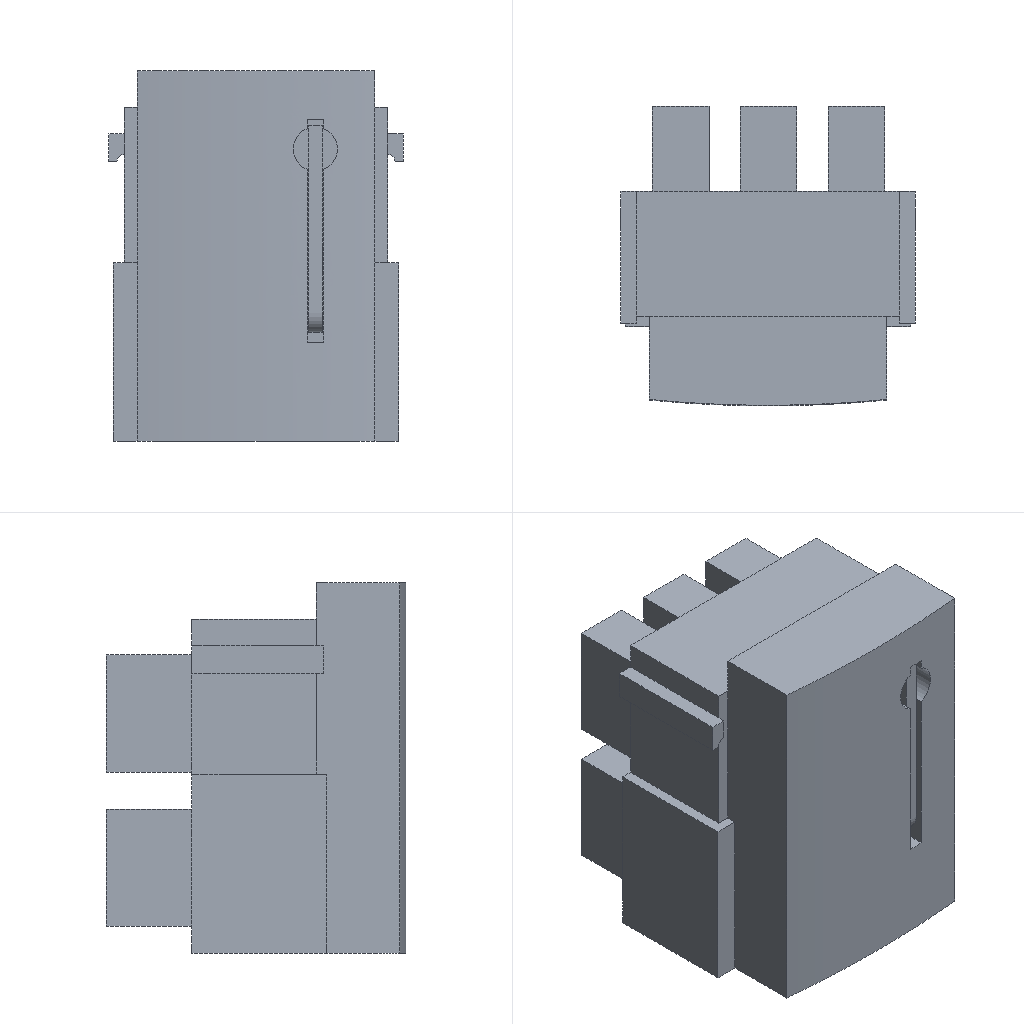Simulation study | abaqus
Set-up summary:
category,name,step,type,value,unit,region
solver,abaqus,,Abaqus/CAE 2024
units,mm-N-s-tonne (MPa),,inferred,E=200000 density=7.8e-09
analysis,Step-1,,dynamic implicit,time_period=0.02
analysis,Step-2,,dynamic implicit,time_period=0.02
mesh,nodes,,,214940
mesh,elements,,,173322
element_type,C3D8R,,,173322
material,Q235,,E,200000
material,Q235,,nu,0.3
material,Q235,,density,7.8e-09
material,Q235,,behaviors,damping
section,Q235,,solid section,,,_PickedSet41
bc,BC-1,initial,encastre,[dofs=ENCASTRE],,_PickedSet4
bc,BC-2,Step-1,acceleration,"-1 [dofs=rx,ry,rz,x,y,z n=6]",,_PickedSet14
bc,BC-1,Step-2,encastre,[dofs=ENCASTRE],,_PickedSet4
Abaqus input file, long lists of numbers shortened:
*Heading
** Job name: deck Model name: 0428-Copy
** Generated by: Abaqus/CAE 2024
*Preprint, echo=NO, model=NO, history=NO, contact=NO
**
** PARTS
**
*Part, name=duanluqi
*Node
      1,   188.98,           0.,   78.818
      2,   188.98,         16.5,   78.818
** (214938 more lines like these left out)
*Element, type=C3D8R
   1,    564,  12340,  99771,  10843,      1,    360,  10483,    396
   2,  12340,  12341,  99772,  99771,    360,    361,  10484,  10483
** (173320 more lines like these left out)
*Nset, nset=_PickedSet41, internal, generate
      1,  214940,       1
*Elset, elset=_PickedSet41, internal, generate
      1,  173322,       1
** Section: Section-1
*Solid Section, elset=_PickedSet41, material=Q235
,
*End Part
**
**
** ASSEMBLY
**
*Assembly, name=Assembly
**
*Instance, name=duanluqi-1, part=duanluqi
*End Instance
**
*Nset, nset=_PickedSet4, internal, instance=duanluqi-1
    10,    11,    12,    13,    19,    22,    47,    48,   109,   110,   113,   115,   116,   117,   441,   442
   443,   444,   445,   446,   447,   448,   449,   450,   451,   452,   453,   454,   455,   456,   457,   458
** (262 more lines like these left out)
*Elset, elset=_PickedSet4, internal, instance=duanluqi-1
  5601,  5602,  5603,  5604,  5605,  5606,  5607,  5608,  5609,  5610,  5611,  5612,  5613,  5614,  5615,  5616
  5617,  5618,  5619,  5620,  5621,  5622,  5623,  5624,  5625,  5626,  5627,  5628,  5629,  5630,  5631,  5632
** (253 more lines like these left out)
*Nset, nset=_PickedSet14, internal, instance=duanluqi-1
    26,    27,    40,    41,    43,   319,   320,  1240,  1241,  1242,  1243,  1244,  1245,  1246,  1247,  1248
  1249,  1250,  1251,  1252,  1253,  1254,  1255,  1256,  1257,  1258,  1259,  1260,  1261,  1262,  1263,  1264
** (55 more lines like these left out)
*Elset, elset=_PickedSet14, internal, instance=duanluqi-1
  29009,  29010,  29011,  29012,  29013,  29014,  29015,  29016,  29017,  29018,  29019,  29020,  29021,  29022,  29023,  29024
  29025,  29026,  29027,  29028,  29029,  29030,  29031,  29032,  29033,  29034,  29035,  29036,  29037,  29038,  29039,  29040
** (50 more lines like these left out)
*Elset, elset=__PickedSurf12_S4, internal, instance=duanluqi-1
   5922,   6020,   6118,   6216,   6314,   6412,   6510,   6608,   6706,   6804,   6902,   7000,   7098,   7196,   7294,   7392
   7490,   7588,   7686,   7784,   7882,   7980,   8078,   8176,   8274,   8372,   8470,   8568,   8666,   8764,   8862,   8960
** (26 more lines like these left out)
*Elset, elset=__PickedSurf12_S2, internal, instance=duanluqi-1
 127371, 127372, 127373, 127374, 127375, 127376, 127377, 127378, 127379, 127380, 127381, 127382, 127383, 127384, 127385, 127386
 127387, 127388, 127389, 127390, 127391, 127392, 127393, 127394, 127395, 127396, 127397, 127398, 127399, 127400, 127401, 127402
** (54 more lines like these left out)
*Elset, elset=__PickedSurf12_S5, internal, instance=duanluqi-1
 29009, 29010, 29011, 29012, 29013, 29014, 29015, 29016, 29017, 29018, 29019, 29020, 29021, 29022, 29023, 29024
 29025, 29026, 29027, 29028, 29029, 29030, 29031, 29032, 29033, 29034, 29035, 29036, 29037, 29038, 29039, 29040
** (10 more lines like these left out)
*Surface, type=ELEMENT, name=_PickedSurf12, internal
__PickedSurf12_S4, S4
__PickedSurf12_S2, S2
__PickedSurf12_S5, S5
*End Assembly
*Amplitude, name=Amp-1
             0.,              0.,          0.0057,              0.,           0.019,         392000.,          0.0191,              0.
           0.02,              0.
**
** MATERIALS
**
*Material, name=Q235
*Damping, alpha=0.3132, beta=7.94e-06
*Density
 7.8e-09,
*Elastic
200000., 0.3
**
** INTERACTION PROPERTIES
**
*Surface Interaction, name=IntProp-1
1.,
*Friction, slip tolerance=0.005
 0.1,
*Surface Behavior, pressure-overclosure=HARD
**
** BOUNDARY CONDITIONS
**
** Name: BC-1 Type: Symmetry/Antisymmetry/Encastre
*Boundary
_PickedSet4, ENCASTRE
** ----------------------------------------------------------------
**
** STEP: Step-1
**
*Step, name=Step-1, nlgeom=NO, inc=1000
*Dynamic
0.002,0.02,2e-07
**
** BOUNDARY CONDITIONS
**
** Name: BC-2 Type: Acceleration/Angular acceleration
*Boundary, amplitude=Amp-1, type=ACCELERATION
_PickedSet14, 1, 1
_PickedSet14, 2, 2
_PickedSet14, 3, 3, -1.
_PickedSet14, 4, 4
_PickedSet14, 5, 5
_PickedSet14, 6, 6
**
** OUTPUT REQUESTS
**
*Restart, write, number interval=1, time marks=NO
**
** FIELD OUTPUT: F-Output-1
**
*Output, field, variable=PRESELECT, number interval=20, time marks=NO
**
** HISTORY OUTPUT: H-Output-1
**
*Output, history, variable=PRESELECT, number interval=200, time marks=NO
*End Step
** ----------------------------------------------------------------
**
** STEP: Step-2
**
*Step, name=Step-2, nlgeom=NO
*Dynamic
0.002,0.02,2e-07
**
** BOUNDARY CONDITIONS
**
** Name: BC-1 Type: Symmetry/Antisymmetry/Encastre
*Boundary, op=NEW
_PickedSet4, ENCASTRE
** Name: BC-2 Type: Acceleration/Angular acceleration
*Boundary, op=NEW
**
** OUTPUT REQUESTS
**
*Restart, write, frequency=0
**
** FIELD OUTPUT: F-Output-1
**
*Output, field, variable=PRESELECT, number interval=20, time marks=NO
**
** HISTORY OUTPUT: H-Output-1
**
*Output, history, variable=PRESELECT, number interval=200, time marks=NO
*End Step
Results summary:
result,odb.job_status,,,JOB_STATUS_COMPLETED_SUCCESSFULLY,"consistent, unstated (Abaqus has no unit system)"
result,steps[0].procedure,Step-1,,*DYNAMIC,"consistent, unstated (Abaqus has no unit system)"
result,steps[0].time_period,Step-1,,0.02,"consistent, unstated (Abaqus has no unit system)"
result,steps[0].n_frames,Step-1,,11,"consistent, unstated (Abaqus has no unit system)"
result,steps[0].last_frame.id,Step-1,,10,"consistent, unstated (Abaqus has no unit system)"
result,steps[0].last_frame.value,Step-1,,0.02,"consistent, unstated (Abaqus has no unit system)"
result,steps[0].last_frame.description,Step-1,,Increment     10: Step Time =   2.0000E-02,"consistent, unstated (Abaqus has no unit system)"
result,steps[0].completed,Step-1,,True,"consistent, unstated (Abaqus has no unit system)"
result,steps[0].max_U_magnitude,Step-1,,15.022,"consistent, unstated (Abaqus has no unit system)"
result,steps[0].max_S_mises,Step-1,,65926.5,"consistent, unstated (Abaqus has no unit system)"
result,steps[0].RF_sum[1],Step-1,,-5.738,"consistent, unstated (Abaqus has no unit system)"
result,steps[0].RF_sum[2],Step-1,,-419.457,"consistent, unstated (Abaqus has no unit system)"
result,steps[0].RF_sum[3],Step-1,,-1775.8,"consistent, unstated (Abaqus has no unit system)"
result,steps[1].procedure,Step-2,,*DYNAMIC,"consistent, unstated (Abaqus has no unit system)"
result,steps[1].time_period,Step-2,,0.02,"consistent, unstated (Abaqus has no unit system)"
result,steps[1].n_frames,Step-2,,17,"consistent, unstated (Abaqus has no unit system)"
result,steps[1].last_frame.id,Step-2,,55,"consistent, unstated (Abaqus has no unit system)"
result,steps[1].last_frame.value,Step-2,,0.02,"consistent, unstated (Abaqus has no unit system)"
result,steps[1].last_frame.description,Step-2,,Increment     55: Step Time =   2.0000E-02,"consistent, unstated (Abaqus has no unit system)"
result,steps[1].completed,Step-2,,True,"consistent, unstated (Abaqus has no unit system)"
result,steps[1].max_U_magnitude,Step-2,,1.947,"consistent, unstated (Abaqus has no unit system)"
result,steps[1].max_S_mises,Step-2,,970.12,"consistent, unstated (Abaqus has no unit system)"
result,steps[1].RF_sum[1],Step-2,,19433.6,"consistent, unstated (Abaqus has no unit system)"
result,steps[1].RF_sum[2],Step-2,,-796124,"consistent, unstated (Abaqus has no unit system)"
result,steps[1].RF_sum[3],Step-2,,-1.25034e+06,"consistent, unstated (Abaqus has no unit system)"